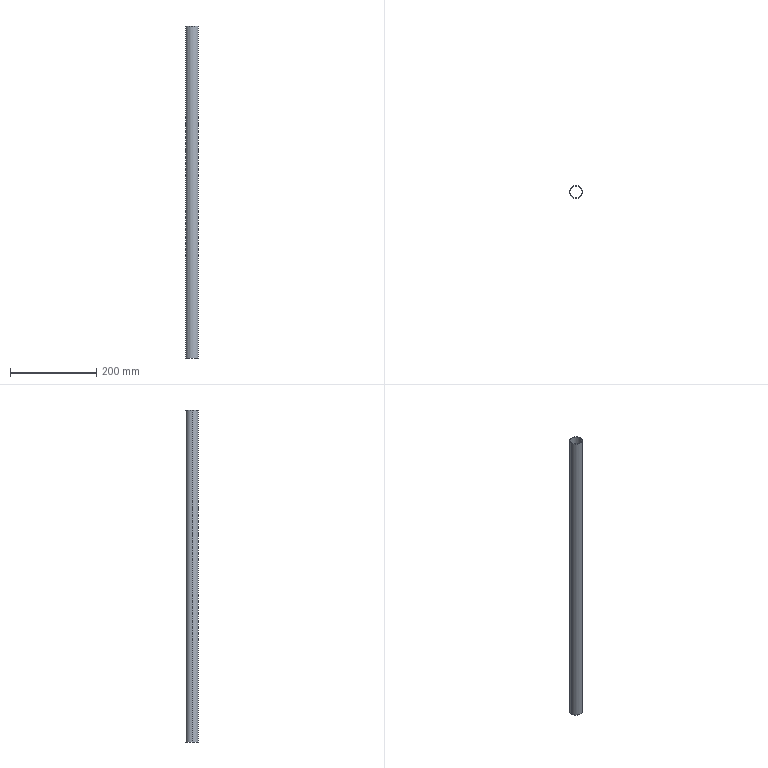Part | STEP file | Guide roller housing 3 | 1 solid | 6 faces | box 29.5 x 29.5 x 770 mm | volume 45363 mm3 | cylinder 4 | plane 2 | commonest cylinder face diameters 28.2 x2 29.5 x2
STEP:
#1=CARTESIAN_POINT('',(0.,0.,0.));
#2=DIRECTION('',(0.,0.,1.));
#3=DIRECTION('',(1.,0.,0.));
#4=AXIS2_PLACEMENT_3D('',#1,#2,#3);
#5=CARTESIAN_POINT('',(14.75,0.,0.));
#6=VERTEX_POINT('',#5);
#7=CARTESIAN_POINT('',(-14.75,0.,0.));
#8=VERTEX_POINT('',#7);
#9=CARTESIAN_POINT('',(0.,0.,0.));
#10=DIRECTION('',(0.,0.,1.));
#11=DIRECTION('',(1.,0.,0.));
#12=AXIS2_PLACEMENT_3D('',#9,#10,#11);
#13=CIRCLE('',#12,14.75);
#14=CARTESIAN_POINT('',(0.,0.,0.));
#15=DIRECTION('',(0.,0.,1.));
#16=DIRECTION('',(1.,0.,0.));
#17=AXIS2_PLACEMENT_3D('',#14,#15,#16);
#18=CYLINDRICAL_SURFACE('',#17,14.75);
#19=CARTESIAN_POINT('',(0.,0.));
#20=DIRECTION('',(1.,0.));
#21=VECTOR('',#20,1.);
#22=LINE('',#19,#21);
#23=(GEOMETRIC_REPRESENTATION_CONTEXT(2)PARAMETRIC_REPRESENTATION_CONTEXT()REPRESENTATION_CONTEXT('',''));
#24=DEFINITIONAL_REPRESENTATION('',(#22),#23);
#25=PCURVE('',#18,#24);
#26=CARTESIAN_POINT('',(0.,0.,0.));
#27=DIRECTION('',(0.,0.,-1.));
#28=DIRECTION('',(-1.,0.,0.));
#29=AXIS2_PLACEMENT_3D('',#26,#27,#28);
#30=PLANE('',#29);
#31=CARTESIAN_POINT('',(-14.75,0.));
#32=CARTESIAN_POINT('',(-14.75,25.548));
#33=CARTESIAN_POINT('',(7.375,12.774));
#34=CARTESIAN_POINT('',(29.5,0.));
#35=CARTESIAN_POINT('',(7.375,-12.774));
#36=CARTESIAN_POINT('',(-14.75,-25.548));
#37=CARTESIAN_POINT('',(-14.75,0.));
#38=(BOUNDED_CURVE()B_SPLINE_CURVE(2,(#31,#32,#33,#34,#35,#36,#37),.UNSPECIFIED.,.T.,.F.)B_SPLINE_CURVE_WITH_KNOTS((1,2,2,2,2,1),(-2.094,0.,2.094,4.189,6.283,8.378),.UNSPECIFIED.)CURVE()GEOMETRIC_REPRESENTATION_ITEM()RATIONAL_B_SPLINE_CURVE((1.,0.5,1.,0.5,1.,0.5,1.))REPRESENTATION_ITEM(''));
#39=(GEOMETRIC_REPRESENTATION_CONTEXT(2)PARAMETRIC_REPRESENTATION_CONTEXT()REPRESENTATION_CONTEXT('',''));
#40=DEFINITIONAL_REPRESENTATION('',(#38),#39);
#41=PCURVE('',#30,#40);
#42=SURFACE_CURVE('',#13,(#25,#41),.PCURVE_S1.);
#43=EDGE_CURVE('',#6,#8,#42,.T.);
#44=ORIENTED_EDGE('',*,*,#43,.T.);
#45=CARTESIAN_POINT('',(-14.75,0.,770.));
#46=VERTEX_POINT('',#45);
#47=CARTESIAN_POINT('',(-14.75,0.,0.));
#48=DIRECTION('',(0.,0.,1.));
#49=VECTOR('',#48,1.);
#50=LINE('',#47,#49);
#51=CARTESIAN_POINT('',(3.142,0.));
#52=DIRECTION('',(0.,1.));
#53=VECTOR('',#52,1.);
#54=LINE('',#51,#53);
#55=(GEOMETRIC_REPRESENTATION_CONTEXT(2)PARAMETRIC_REPRESENTATION_CONTEXT()REPRESENTATION_CONTEXT('',''));
#56=DEFINITIONAL_REPRESENTATION('',(#54),#55);
#57=PCURVE('',#18,#56);
#58=CARTESIAN_POINT('',(0.,0.,0.));
#59=DIRECTION('',(0.,0.,1.));
#60=DIRECTION('',(1.,0.,0.));
#61=AXIS2_PLACEMENT_3D('',#58,#59,#60);
#62=CYLINDRICAL_SURFACE('',#61,14.75);
#63=CARTESIAN_POINT('',(3.142,0.));
#64=DIRECTION('',(0.,1.));
#65=VECTOR('',#64,1.);
#66=LINE('',#63,#65);
#67=(GEOMETRIC_REPRESENTATION_CONTEXT(2)PARAMETRIC_REPRESENTATION_CONTEXT()REPRESENTATION_CONTEXT('',''));
#68=DEFINITIONAL_REPRESENTATION('',(#66),#67);
#69=PCURVE('',#62,#68);
#70=SURFACE_CURVE('',#50,(#57,#69),.PCURVE_S1.);
#71=EDGE_CURVE('',#8,#46,#70,.T.);
#72=ORIENTED_EDGE('',*,*,#71,.T.);
#73=CARTESIAN_POINT('',(14.75,0.,770.));
#74=VERTEX_POINT('',#73);
#75=CARTESIAN_POINT('',(0.,0.,770.));
#76=DIRECTION('',(0.,0.,-1.));
#77=DIRECTION('',(1.,0.,0.));
#78=AXIS2_PLACEMENT_3D('',#75,#76,#77);
#79=CIRCLE('',#78,14.75);
#80=CARTESIAN_POINT('',(6.283,770.));
#81=DIRECTION('',(-1.,0.));
#82=VECTOR('',#81,1.);
#83=LINE('',#80,#82);
#84=(GEOMETRIC_REPRESENTATION_CONTEXT(2)PARAMETRIC_REPRESENTATION_CONTEXT()REPRESENTATION_CONTEXT('',''));
#85=DEFINITIONAL_REPRESENTATION('',(#83),#84);
#86=PCURVE('',#18,#85);
#87=CARTESIAN_POINT('',(0.,0.,770.));
#88=DIRECTION('',(0.,0.,-1.));
#89=DIRECTION('',(-1.,0.,0.));
#90=AXIS2_PLACEMENT_3D('',#87,#88,#89);
#91=PLANE('',#90);
#92=CARTESIAN_POINT('',(0.,0.));
#93=DIRECTION('',(-1.,0.));
#94=AXIS2_PLACEMENT_2D('',#92,#93);
#95=CIRCLE('',#94,14.75);
#96=(GEOMETRIC_REPRESENTATION_CONTEXT(2)PARAMETRIC_REPRESENTATION_CONTEXT()REPRESENTATION_CONTEXT('',''));
#97=DEFINITIONAL_REPRESENTATION('',(#95),#96);
#98=PCURVE('',#91,#97);
#99=SURFACE_CURVE('',#79,(#86,#98),.PCURVE_S1.);
#100=EDGE_CURVE('',#46,#74,#99,.T.);
#101=ORIENTED_EDGE('',*,*,#100,.T.);
#102=CARTESIAN_POINT('',(14.75,0.,0.));
#103=DIRECTION('',(0.,0.,1.));
#104=VECTOR('',#103,1.);
#105=LINE('',#102,#104);
#106=CARTESIAN_POINT('',(0.,0.));
#107=DIRECTION('',(0.,1.));
#108=VECTOR('',#107,1.);
#109=LINE('',#106,#108);
#110=(GEOMETRIC_REPRESENTATION_CONTEXT(2)PARAMETRIC_REPRESENTATION_CONTEXT()REPRESENTATION_CONTEXT('',''));
#111=DEFINITIONAL_REPRESENTATION('',(#109),#110);
#112=PCURVE('',#18,#111);
#113=CARTESIAN_POINT('',(6.283,0.));
#114=DIRECTION('',(0.,1.));
#115=VECTOR('',#114,1.);
#116=LINE('',#113,#115);
#117=(GEOMETRIC_REPRESENTATION_CONTEXT(2)PARAMETRIC_REPRESENTATION_CONTEXT()REPRESENTATION_CONTEXT('',''));
#118=DEFINITIONAL_REPRESENTATION('',(#116),#117);
#119=PCURVE('',#62,#118);
#120=SURFACE_CURVE('',#105,(#112,#119),.PCURVE_S1.);
#121=EDGE_CURVE('',#6,#74,#120,.T.);
#122=ORIENTED_EDGE('',*,*,#121,.F.);
#123=EDGE_LOOP('',(#44,#72,#101,#122));
#124=FACE_BOUND('',#123,.T.);
#125=ADVANCED_FACE('',(#124),#18,.T.);
#126=CARTESIAN_POINT('',(14.1,0.,0.));
#127=VERTEX_POINT('',#126);
#128=CARTESIAN_POINT('',(14.1,0.,770.));
#129=VERTEX_POINT('',#128);
#130=CARTESIAN_POINT('',(14.1,0.,0.));
#131=DIRECTION('',(0.,0.,1.));
#132=VECTOR('',#131,1.);
#133=LINE('',#130,#132);
#134=CARTESIAN_POINT('',(0.,0.,0.));
#135=DIRECTION('',(0.,0.,1.));
#136=DIRECTION('',(1.,0.,0.));
#137=AXIS2_PLACEMENT_3D('',#134,#135,#136);
#138=CYLINDRICAL_SURFACE('',#137,14.1);
#139=CARTESIAN_POINT('',(6.283,0.));
#140=DIRECTION('',(0.,1.));
#141=VECTOR('',#140,1.);
#142=LINE('',#139,#141);
#143=(GEOMETRIC_REPRESENTATION_CONTEXT(2)PARAMETRIC_REPRESENTATION_CONTEXT()REPRESENTATION_CONTEXT('',''));
#144=DEFINITIONAL_REPRESENTATION('',(#142),#143);
#145=PCURVE('',#138,#144);
#146=CARTESIAN_POINT('',(0.,0.,0.));
#147=DIRECTION('',(0.,0.,1.));
#148=DIRECTION('',(1.,0.,0.));
#149=AXIS2_PLACEMENT_3D('',#146,#147,#148);
#150=CYLINDRICAL_SURFACE('',#149,14.1);
#151=CARTESIAN_POINT('',(0.,0.));
#152=DIRECTION('',(0.,1.));
#153=VECTOR('',#152,1.);
#154=LINE('',#151,#153);
#155=(GEOMETRIC_REPRESENTATION_CONTEXT(2)PARAMETRIC_REPRESENTATION_CONTEXT()REPRESENTATION_CONTEXT('',''));
#156=DEFINITIONAL_REPRESENTATION('',(#154),#155);
#157=PCURVE('',#150,#156);
#158=SURFACE_CURVE('',#133,(#145,#157),.PCURVE_S1.);
#159=EDGE_CURVE('',#127,#129,#158,.T.);
#160=ORIENTED_EDGE('',*,*,#159,.T.);
#161=CARTESIAN_POINT('',(-14.1,0.,770.));
#162=VERTEX_POINT('',#161);
#163=CARTESIAN_POINT('',(0.,0.,770.));
#164=DIRECTION('',(0.,0.,1.));
#165=DIRECTION('',(1.,0.,0.));
#166=AXIS2_PLACEMENT_3D('',#163,#164,#165);
#167=CIRCLE('',#166,14.1);
#168=CARTESIAN_POINT('',(0.,770.));
#169=DIRECTION('',(1.,0.));
#170=VECTOR('',#169,1.);
#171=LINE('',#168,#170);
#172=(GEOMETRIC_REPRESENTATION_CONTEXT(2)PARAMETRIC_REPRESENTATION_CONTEXT()REPRESENTATION_CONTEXT('',''));
#173=DEFINITIONAL_REPRESENTATION('',(#171),#172);
#174=PCURVE('',#138,#173);
#175=CARTESIAN_POINT('',(-14.1,0.));
#176=CARTESIAN_POINT('',(-14.1,24.422));
#177=CARTESIAN_POINT('',(7.05,12.211));
#178=CARTESIAN_POINT('',(28.2,0.));
#179=CARTESIAN_POINT('',(7.05,-12.211));
#180=CARTESIAN_POINT('',(-14.1,-24.422));
#181=CARTESIAN_POINT('',(-14.1,0.));
#182=(BOUNDED_CURVE()B_SPLINE_CURVE(2,(#175,#176,#177,#178,#179,#180,#181),.UNSPECIFIED.,.T.,.F.)B_SPLINE_CURVE_WITH_KNOTS((1,2,2,2,2,1),(-2.094,0.,2.094,4.189,6.283,8.378),.UNSPECIFIED.)CURVE()GEOMETRIC_REPRESENTATION_ITEM()RATIONAL_B_SPLINE_CURVE((1.,0.5,1.,0.5,1.,0.5,1.))REPRESENTATION_ITEM(''));
#183=(GEOMETRIC_REPRESENTATION_CONTEXT(2)PARAMETRIC_REPRESENTATION_CONTEXT()REPRESENTATION_CONTEXT('',''));
#184=DEFINITIONAL_REPRESENTATION('',(#182),#183);
#185=PCURVE('',#91,#184);
#186=SURFACE_CURVE('',#167,(#174,#185),.PCURVE_S1.);
#187=EDGE_CURVE('',#162,#129,#186,.T.);
#188=ORIENTED_EDGE('',*,*,#187,.F.);
#189=CARTESIAN_POINT('',(-14.1,0.,0.));
#190=VERTEX_POINT('',#189);
#191=CARTESIAN_POINT('',(-14.1,0.,0.));
#192=DIRECTION('',(0.,0.,1.));
#193=VECTOR('',#192,1.);
#194=LINE('',#191,#193);
#195=CARTESIAN_POINT('',(3.142,0.));
#196=DIRECTION('',(0.,1.));
#197=VECTOR('',#196,1.);
#198=LINE('',#195,#197);
#199=(GEOMETRIC_REPRESENTATION_CONTEXT(2)PARAMETRIC_REPRESENTATION_CONTEXT()REPRESENTATION_CONTEXT('',''));
#200=DEFINITIONAL_REPRESENTATION('',(#198),#199);
#201=PCURVE('',#138,#200);
#202=CARTESIAN_POINT('',(3.142,0.));
#203=DIRECTION('',(0.,1.));
#204=VECTOR('',#203,1.);
#205=LINE('',#202,#204);
#206=(GEOMETRIC_REPRESENTATION_CONTEXT(2)PARAMETRIC_REPRESENTATION_CONTEXT()REPRESENTATION_CONTEXT('',''));
#207=DEFINITIONAL_REPRESENTATION('',(#205),#206);
#208=PCURVE('',#150,#207);
#209=SURFACE_CURVE('',#194,(#201,#208),.PCURVE_S1.);
#210=EDGE_CURVE('',#190,#162,#209,.T.);
#211=ORIENTED_EDGE('',*,*,#210,.F.);
#212=CARTESIAN_POINT('',(0.,0.,0.));
#213=DIRECTION('',(0.,0.,1.));
#214=DIRECTION('',(1.,0.,0.));
#215=AXIS2_PLACEMENT_3D('',#212,#213,#214);
#216=CIRCLE('',#215,14.1);
#217=CARTESIAN_POINT('',(0.,0.));
#218=DIRECTION('',(1.,0.));
#219=VECTOR('',#218,1.);
#220=LINE('',#217,#219);
#221=(GEOMETRIC_REPRESENTATION_CONTEXT(2)PARAMETRIC_REPRESENTATION_CONTEXT()REPRESENTATION_CONTEXT('',''));
#222=DEFINITIONAL_REPRESENTATION('',(#220),#221);
#223=PCURVE('',#138,#222);
#224=CARTESIAN_POINT('',(-14.1,0.));
#225=CARTESIAN_POINT('',(-14.1,24.422));
#226=CARTESIAN_POINT('',(7.05,12.211));
#227=CARTESIAN_POINT('',(28.2,0.));
#228=CARTESIAN_POINT('',(7.05,-12.211));
#229=CARTESIAN_POINT('',(-14.1,-24.422));
#230=CARTESIAN_POINT('',(-14.1,0.));
#231=(BOUNDED_CURVE()B_SPLINE_CURVE(2,(#224,#225,#226,#227,#228,#229,#230),.UNSPECIFIED.,.T.,.F.)B_SPLINE_CURVE_WITH_KNOTS((1,2,2,2,2,1),(-2.094,0.,2.094,4.189,6.283,8.378),.UNSPECIFIED.)CURVE()GEOMETRIC_REPRESENTATION_ITEM()RATIONAL_B_SPLINE_CURVE((1.,0.5,1.,0.5,1.,0.5,1.))REPRESENTATION_ITEM(''));
#232=(GEOMETRIC_REPRESENTATION_CONTEXT(2)PARAMETRIC_REPRESENTATION_CONTEXT()REPRESENTATION_CONTEXT('',''));
#233=DEFINITIONAL_REPRESENTATION('',(#231),#232);
#234=PCURVE('',#30,#233);
#235=SURFACE_CURVE('',#216,(#223,#234),.PCURVE_S1.);
#236=EDGE_CURVE('',#190,#127,#235,.T.);
#237=ORIENTED_EDGE('',*,*,#236,.T.);
#238=EDGE_LOOP('',(#160,#188,#211,#237));
#239=FACE_BOUND('',#238,.F.);
#240=ADVANCED_FACE('',(#239),#138,.F.);
#241=ORIENTED_EDGE('',*,*,#71,.F.);
#242=CARTESIAN_POINT('',(0.,0.,0.));
#243=DIRECTION('',(0.,0.,1.));
#244=DIRECTION('',(1.,0.,0.));
#245=AXIS2_PLACEMENT_3D('',#242,#243,#244);
#246=CIRCLE('',#245,14.75);
#247=CARTESIAN_POINT('',(0.,0.));
#248=DIRECTION('',(1.,0.));
#249=VECTOR('',#248,1.);
#250=LINE('',#247,#249);
#251=(GEOMETRIC_REPRESENTATION_CONTEXT(2)PARAMETRIC_REPRESENTATION_CONTEXT()REPRESENTATION_CONTEXT('',''));
#252=DEFINITIONAL_REPRESENTATION('',(#250),#251);
#253=PCURVE('',#62,#252);
#254=CARTESIAN_POINT('',(-14.75,0.));
#255=CARTESIAN_POINT('',(-14.75,25.548));
#256=CARTESIAN_POINT('',(7.375,12.774));
#257=CARTESIAN_POINT('',(29.5,0.));
#258=CARTESIAN_POINT('',(7.375,-12.774));
#259=CARTESIAN_POINT('',(-14.75,-25.548));
#260=CARTESIAN_POINT('',(-14.75,0.));
#261=(BOUNDED_CURVE()B_SPLINE_CURVE(2,(#254,#255,#256,#257,#258,#259,#260),.UNSPECIFIED.,.T.,.F.)B_SPLINE_CURVE_WITH_KNOTS((1,2,2,2,2,1),(-2.094,0.,2.094,4.189,6.283,8.378),.UNSPECIFIED.)CURVE()GEOMETRIC_REPRESENTATION_ITEM()RATIONAL_B_SPLINE_CURVE((1.,0.5,1.,0.5,1.,0.5,1.))REPRESENTATION_ITEM(''));
#262=(GEOMETRIC_REPRESENTATION_CONTEXT(2)PARAMETRIC_REPRESENTATION_CONTEXT()REPRESENTATION_CONTEXT('',''));
#263=DEFINITIONAL_REPRESENTATION('',(#261),#262);
#264=PCURVE('',#30,#263);
#265=SURFACE_CURVE('',#246,(#253,#264),.PCURVE_S1.);
#266=EDGE_CURVE('',#8,#6,#265,.T.);
#267=ORIENTED_EDGE('',*,*,#266,.T.);
#268=ORIENTED_EDGE('',*,*,#121,.T.);
#269=CARTESIAN_POINT('',(0.,0.,770.));
#270=DIRECTION('',(0.,0.,-1.));
#271=DIRECTION('',(1.,0.,0.));
#272=AXIS2_PLACEMENT_3D('',#269,#270,#271);
#273=CIRCLE('',#272,14.75);
#274=CARTESIAN_POINT('',(6.283,770.));
#275=DIRECTION('',(-1.,0.));
#276=VECTOR('',#275,1.);
#277=LINE('',#274,#276);
#278=(GEOMETRIC_REPRESENTATION_CONTEXT(2)PARAMETRIC_REPRESENTATION_CONTEXT()REPRESENTATION_CONTEXT('',''));
#279=DEFINITIONAL_REPRESENTATION('',(#277),#278);
#280=PCURVE('',#62,#279);
#281=CARTESIAN_POINT('',(0.,0.));
#282=DIRECTION('',(-1.,0.));
#283=AXIS2_PLACEMENT_2D('',#281,#282);
#284=CIRCLE('',#283,14.75);
#285=(GEOMETRIC_REPRESENTATION_CONTEXT(2)PARAMETRIC_REPRESENTATION_CONTEXT()REPRESENTATION_CONTEXT('',''));
#286=DEFINITIONAL_REPRESENTATION('',(#284),#285);
#287=PCURVE('',#91,#286);
#288=SURFACE_CURVE('',#273,(#280,#287),.PCURVE_S1.);
#289=EDGE_CURVE('',#74,#46,#288,.T.);
#290=ORIENTED_EDGE('',*,*,#289,.T.);
#291=EDGE_LOOP('',(#241,#267,#268,#290));
#292=FACE_BOUND('',#291,.T.);
#293=ADVANCED_FACE('',(#292),#62,.T.);
#294=CARTESIAN_POINT('',(0.,0.,0.));
#295=DIRECTION('',(0.,0.,1.));
#296=DIRECTION('',(1.,0.,0.));
#297=AXIS2_PLACEMENT_3D('',#294,#295,#296);
#298=CIRCLE('',#297,14.1);
#299=CARTESIAN_POINT('',(-14.1,0.));
#300=CARTESIAN_POINT('',(-14.1,24.422));
#301=CARTESIAN_POINT('',(7.05,12.211));
#302=CARTESIAN_POINT('',(28.2,0.));
#303=CARTESIAN_POINT('',(7.05,-12.211));
#304=CARTESIAN_POINT('',(-14.1,-24.422));
#305=CARTESIAN_POINT('',(-14.1,0.));
#306=(BOUNDED_CURVE()B_SPLINE_CURVE(2,(#299,#300,#301,#302,#303,#304,#305),.UNSPECIFIED.,.T.,.F.)B_SPLINE_CURVE_WITH_KNOTS((1,2,2,2,2,1),(-2.094,0.,2.094,4.189,6.283,8.378),.UNSPECIFIED.)CURVE()GEOMETRIC_REPRESENTATION_ITEM()RATIONAL_B_SPLINE_CURVE((1.,0.5,1.,0.5,1.,0.5,1.))REPRESENTATION_ITEM(''));
#307=(GEOMETRIC_REPRESENTATION_CONTEXT(2)PARAMETRIC_REPRESENTATION_CONTEXT()REPRESENTATION_CONTEXT('',''));
#308=DEFINITIONAL_REPRESENTATION('',(#306),#307);
#309=PCURVE('',#30,#308);
#310=CARTESIAN_POINT('',(0.,0.));
#311=DIRECTION('',(1.,0.));
#312=VECTOR('',#311,1.);
#313=LINE('',#310,#312);
#314=(GEOMETRIC_REPRESENTATION_CONTEXT(2)PARAMETRIC_REPRESENTATION_CONTEXT()REPRESENTATION_CONTEXT('',''));
#315=DEFINITIONAL_REPRESENTATION('',(#313),#314);
#316=PCURVE('',#150,#315);
#317=SURFACE_CURVE('',#298,(#309,#316),.PCURVE_S1.);
#318=EDGE_CURVE('',#127,#190,#317,.T.);
#319=ORIENTED_EDGE('',*,*,#318,.T.);
#320=ORIENTED_EDGE('',*,*,#236,.T.);
#321=EDGE_LOOP('',(#319,#320));
#322=FACE_BOUND('',#321,.T.);
#323=ORIENTED_EDGE('',*,*,#43,.F.);
#324=ORIENTED_EDGE('',*,*,#266,.F.);
#325=EDGE_LOOP('',(#323,#324));
#326=FACE_BOUND('',#325,.T.);
#327=ADVANCED_FACE('',(#322,#326),#30,.T.);
#328=CARTESIAN_POINT('',(0.,0.,770.));
#329=DIRECTION('',(0.,0.,1.));
#330=DIRECTION('',(1.,0.,0.));
#331=AXIS2_PLACEMENT_3D('',#328,#329,#330);
#332=CIRCLE('',#331,14.1);
#333=CARTESIAN_POINT('',(-14.1,0.));
#334=CARTESIAN_POINT('',(-14.1,24.422));
#335=CARTESIAN_POINT('',(7.05,12.211));
#336=CARTESIAN_POINT('',(28.2,0.));
#337=CARTESIAN_POINT('',(7.05,-12.211));
#338=CARTESIAN_POINT('',(-14.1,-24.422));
#339=CARTESIAN_POINT('',(-14.1,0.));
#340=(BOUNDED_CURVE()B_SPLINE_CURVE(2,(#333,#334,#335,#336,#337,#338,#339),.UNSPECIFIED.,.T.,.F.)B_SPLINE_CURVE_WITH_KNOTS((1,2,2,2,2,1),(-2.094,0.,2.094,4.189,6.283,8.378),.UNSPECIFIED.)CURVE()GEOMETRIC_REPRESENTATION_ITEM()RATIONAL_B_SPLINE_CURVE((1.,0.5,1.,0.5,1.,0.5,1.))REPRESENTATION_ITEM(''));
#341=(GEOMETRIC_REPRESENTATION_CONTEXT(2)PARAMETRIC_REPRESENTATION_CONTEXT()REPRESENTATION_CONTEXT('',''));
#342=DEFINITIONAL_REPRESENTATION('',(#340),#341);
#343=PCURVE('',#91,#342);
#344=CARTESIAN_POINT('',(0.,770.));
#345=DIRECTION('',(1.,0.));
#346=VECTOR('',#345,1.);
#347=LINE('',#344,#346);
#348=(GEOMETRIC_REPRESENTATION_CONTEXT(2)PARAMETRIC_REPRESENTATION_CONTEXT()REPRESENTATION_CONTEXT('',''));
#349=DEFINITIONAL_REPRESENTATION('',(#347),#348);
#350=PCURVE('',#150,#349);
#351=SURFACE_CURVE('',#332,(#343,#350),.PCURVE_S1.);
#352=EDGE_CURVE('',#129,#162,#351,.T.);
#353=ORIENTED_EDGE('',*,*,#352,.F.);
#354=ORIENTED_EDGE('',*,*,#187,.F.);
#355=EDGE_LOOP('',(#353,#354));
#356=FACE_BOUND('',#355,.T.);
#357=ORIENTED_EDGE('',*,*,#289,.F.);
#358=ORIENTED_EDGE('',*,*,#100,.F.);
#359=EDGE_LOOP('',(#357,#358));
#360=FACE_BOUND('',#359,.T.);
#361=ADVANCED_FACE('',(#356,#360),#91,.F.);
#362=ORIENTED_EDGE('',*,*,#352,.F.);
#363=ORIENTED_EDGE('',*,*,#159,.F.);
#364=ORIENTED_EDGE('',*,*,#318,.T.);
#365=ORIENTED_EDGE('',*,*,#210,.T.);
#366=EDGE_LOOP('',(#362,#363,#364,#365));
#367=FACE_BOUND('',#366,.F.);
#368=ADVANCED_FACE('',(#367),#150,.F.);
#369=CLOSED_SHELL('',(#125,#240,#293,#327,#361,#368));
#370=MANIFOLD_SOLID_BREP('',#369);
#371=(LENGTH_UNIT()NAMED_UNIT(*)SI_UNIT(.MILLI.,.METRE.));
#372=UNCERTAINTY_MEASURE_WITH_UNIT(LENGTH_MEASURE(0.0000001),#371,'','');
#373=(NAMED_UNIT(*)PLANE_ANGLE_UNIT()SI_UNIT($,.RADIAN.));
#374=(NAMED_UNIT(*)SI_UNIT($,.STERADIAN.)SOLID_ANGLE_UNIT());
#375=(GEOMETRIC_REPRESENTATION_CONTEXT(3)GLOBAL_UNCERTAINTY_ASSIGNED_CONTEXT((#372))GLOBAL_UNIT_ASSIGNED_CONTEXT((#371,#373,#374))REPRESENTATION_CONTEXT('',''));
#376=ADVANCED_BREP_SHAPE_REPRESENTATION('',(#4,#370),#375);